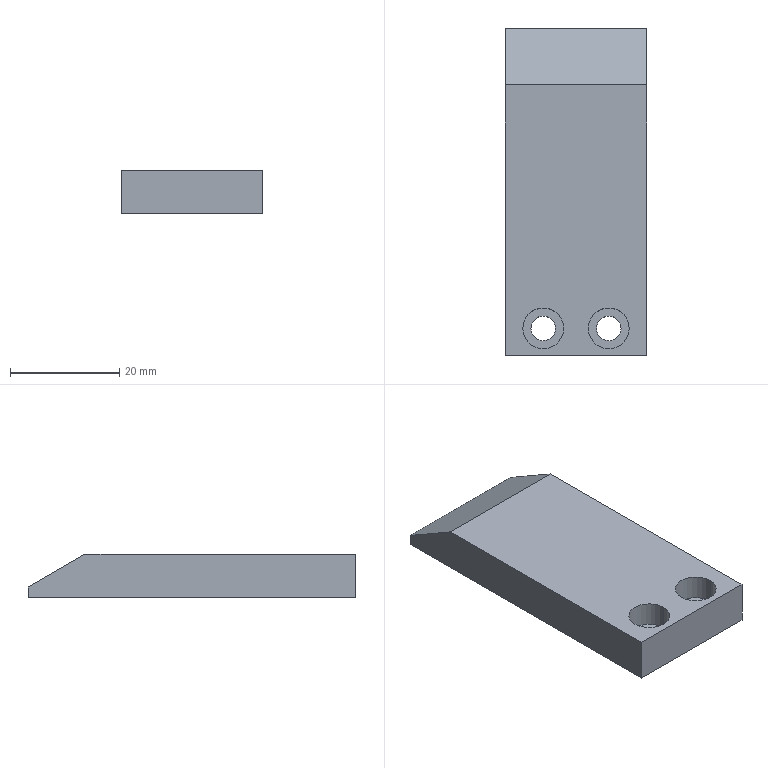Part | STEP file | CA-10-013Pusher Plate | 1 solid | 17 faces | box 26 x 60 x 8 mm | volume 11155 mm3 | plane 9 | cylinder 8 | commonest cylinder face diameters 4.5 x4 7.5 x4
STEP:
#1=CARTESIAN_POINT('',(0.,0.,0.));
#2=DIRECTION('',(0.,0.,1.));
#3=DIRECTION('',(1.,0.,0.));
#4=AXIS2_PLACEMENT_3D('',#1,#2,#3);
#5=CARTESIAN_POINT('',(9.75,-1.,-0.6));
#6=VERTEX_POINT('',#5);
#7=CARTESIAN_POINT('',(9.75,-1.,4.));
#8=VERTEX_POINT('',#7);
#9=CARTESIAN_POINT('',(9.75,-1.,4.));
#10=DIRECTION('',(0.,0.,1.));
#11=VECTOR('',#10,1.);
#12=LINE('',#9,#11);
#13=CARTESIAN_POINT('',(6.,-1.,4.));
#14=DIRECTION('',(0.,0.,1.));
#15=DIRECTION('',(1.,0.,0.));
#16=AXIS2_PLACEMENT_3D('',#13,#14,#15);
#17=CYLINDRICAL_SURFACE('',#16,3.75);
#18=CARTESIAN_POINT('',(6.283,0.));
#19=DIRECTION('',(0.,1.));
#20=VECTOR('',#19,1.);
#21=LINE('',#18,#20);
#22=(GEOMETRIC_REPRESENTATION_CONTEXT(2)PARAMETRIC_REPRESENTATION_CONTEXT()REPRESENTATION_CONTEXT('',''));
#23=DEFINITIONAL_REPRESENTATION('',(#21),#22);
#24=PCURVE('',#17,#23);
#25=CARTESIAN_POINT('',(6.,-1.,4.));
#26=DIRECTION('',(0.,0.,1.));
#27=DIRECTION('',(1.,0.,0.));
#28=AXIS2_PLACEMENT_3D('',#25,#26,#27);
#29=CYLINDRICAL_SURFACE('',#28,3.75);
#30=CARTESIAN_POINT('',(0.,0.));
#31=DIRECTION('',(0.,1.));
#32=VECTOR('',#31,1.);
#33=LINE('',#30,#32);
#34=(GEOMETRIC_REPRESENTATION_CONTEXT(2)PARAMETRIC_REPRESENTATION_CONTEXT()REPRESENTATION_CONTEXT('',''));
#35=DEFINITIONAL_REPRESENTATION('',(#33),#34);
#36=PCURVE('',#29,#35);
#37=SURFACE_CURVE('',#12,(#24,#36),.PCURVE_S1.);
#38=EDGE_CURVE('',#6,#8,#37,.T.);
#39=ORIENTED_EDGE('',*,*,#38,.T.);
#40=CARTESIAN_POINT('',(2.25,-1.,4.));
#41=VERTEX_POINT('',#40);
#42=CARTESIAN_POINT('',(6.,-1.,4.));
#43=DIRECTION('',(0.,0.,1.));
#44=DIRECTION('',(1.,0.,0.));
#45=AXIS2_PLACEMENT_3D('',#42,#43,#44);
#46=CIRCLE('',#45,3.75);
#47=CARTESIAN_POINT('',(0.,0.));
#48=DIRECTION('',(1.,0.));
#49=VECTOR('',#48,1.);
#50=LINE('',#47,#49);
#51=(GEOMETRIC_REPRESENTATION_CONTEXT(2)PARAMETRIC_REPRESENTATION_CONTEXT()REPRESENTATION_CONTEXT('',''));
#52=DEFINITIONAL_REPRESENTATION('',(#50),#51);
#53=PCURVE('',#17,#52);
#54=CARTESIAN_POINT('',(0.,0.,4.));
#55=DIRECTION('',(0.,0.,1.));
#56=DIRECTION('',(1.,0.,0.));
#57=AXIS2_PLACEMENT_3D('',#54,#55,#56);
#58=PLANE('',#57);
#59=CARTESIAN_POINT('',(6.,-1.));
#60=DIRECTION('',(1.,0.));
#61=AXIS2_PLACEMENT_2D('',#59,#60);
#62=CIRCLE('',#61,3.75);
#63=(GEOMETRIC_REPRESENTATION_CONTEXT(2)PARAMETRIC_REPRESENTATION_CONTEXT()REPRESENTATION_CONTEXT('',''));
#64=DEFINITIONAL_REPRESENTATION('',(#62),#63);
#65=PCURVE('',#58,#64);
#66=SURFACE_CURVE('',#46,(#53,#65),.PCURVE_S1.);
#67=EDGE_CURVE('',#41,#8,#66,.T.);
#68=ORIENTED_EDGE('',*,*,#67,.F.);
#69=CARTESIAN_POINT('',(2.25,-1.,-0.6));
#70=VERTEX_POINT('',#69);
#71=CARTESIAN_POINT('',(2.25,-1.,4.));
#72=DIRECTION('',(0.,0.,1.));
#73=VECTOR('',#72,1.);
#74=LINE('',#71,#73);
#75=CARTESIAN_POINT('',(3.142,0.));
#76=DIRECTION('',(0.,1.));
#77=VECTOR('',#76,1.);
#78=LINE('',#75,#77);
#79=(GEOMETRIC_REPRESENTATION_CONTEXT(2)PARAMETRIC_REPRESENTATION_CONTEXT()REPRESENTATION_CONTEXT('',''));
#80=DEFINITIONAL_REPRESENTATION('',(#78),#79);
#81=PCURVE('',#17,#80);
#82=CARTESIAN_POINT('',(3.142,0.));
#83=DIRECTION('',(0.,1.));
#84=VECTOR('',#83,1.);
#85=LINE('',#82,#84);
#86=(GEOMETRIC_REPRESENTATION_CONTEXT(2)PARAMETRIC_REPRESENTATION_CONTEXT()REPRESENTATION_CONTEXT('',''));
#87=DEFINITIONAL_REPRESENTATION('',(#85),#86);
#88=PCURVE('',#29,#87);
#89=SURFACE_CURVE('',#74,(#81,#88),.PCURVE_S1.);
#90=EDGE_CURVE('',#70,#41,#89,.T.);
#91=ORIENTED_EDGE('',*,*,#90,.F.);
#92=CARTESIAN_POINT('',(6.,-1.,-0.6));
#93=DIRECTION('',(0.,0.,1.));
#94=DIRECTION('',(1.,0.,0.));
#95=AXIS2_PLACEMENT_3D('',#92,#93,#94);
#96=CIRCLE('',#95,3.75);
#97=CARTESIAN_POINT('',(0.,-4.6));
#98=DIRECTION('',(1.,0.));
#99=VECTOR('',#98,1.);
#100=LINE('',#97,#99);
#101=(GEOMETRIC_REPRESENTATION_CONTEXT(2)PARAMETRIC_REPRESENTATION_CONTEXT()REPRESENTATION_CONTEXT('',''));
#102=DEFINITIONAL_REPRESENTATION('',(#100),#101);
#103=PCURVE('',#17,#102);
#104=CARTESIAN_POINT('',(8.25,-1.,-0.6));
#105=DIRECTION('',(0.,0.,-1.));
#106=DIRECTION('',(-1.,0.,0.));
#107=AXIS2_PLACEMENT_3D('',#104,#105,#106);
#108=PLANE('',#107);
#109=CARTESIAN_POINT('',(-1.5,0.));
#110=CARTESIAN_POINT('',(-1.5,6.495));
#111=CARTESIAN_POINT('',(4.125,3.248));
#112=CARTESIAN_POINT('',(9.75,0.));
#113=CARTESIAN_POINT('',(4.125,-3.248));
#114=CARTESIAN_POINT('',(-1.5,-6.495));
#115=CARTESIAN_POINT('',(-1.5,0.));
#116=(BOUNDED_CURVE()B_SPLINE_CURVE(2,(#109,#110,#111,#112,#113,#114,#115),.UNSPECIFIED.,.T.,.F.)B_SPLINE_CURVE_WITH_KNOTS((1,2,2,2,2,1),(-2.094,0.,2.094,4.189,6.283,8.378),.UNSPECIFIED.)CURVE()GEOMETRIC_REPRESENTATION_ITEM()RATIONAL_B_SPLINE_CURVE((1.,0.5,1.,0.5,1.,0.5,1.))REPRESENTATION_ITEM(''));
#117=(GEOMETRIC_REPRESENTATION_CONTEXT(2)PARAMETRIC_REPRESENTATION_CONTEXT()REPRESENTATION_CONTEXT('',''));
#118=DEFINITIONAL_REPRESENTATION('',(#116),#117);
#119=PCURVE('',#108,#118);
#120=SURFACE_CURVE('',#96,(#103,#119),.PCURVE_S1.);
#121=EDGE_CURVE('',#70,#6,#120,.T.);
#122=ORIENTED_EDGE('',*,*,#121,.T.);
#123=EDGE_LOOP('',(#39,#68,#91,#122));
#124=FACE_BOUND('',#123,.F.);
#125=ADVANCED_FACE('',(#124),#17,.F.);
#126=CARTESIAN_POINT('',(8.25,-1.,-4.));
#127=VERTEX_POINT('',#126);
#128=CARTESIAN_POINT('',(8.25,-1.,-0.6));
#129=VERTEX_POINT('',#128);
#130=CARTESIAN_POINT('',(8.25,-1.,4.));
#131=DIRECTION('',(0.,0.,1.));
#132=VECTOR('',#131,1.);
#133=LINE('',#130,#132);
#134=CARTESIAN_POINT('',(6.,-1.,4.));
#135=DIRECTION('',(0.,0.,1.));
#136=DIRECTION('',(1.,0.,0.));
#137=AXIS2_PLACEMENT_3D('',#134,#135,#136);
#138=CYLINDRICAL_SURFACE('',#137,2.25);
#139=CARTESIAN_POINT('',(6.283,0.));
#140=DIRECTION('',(0.,1.));
#141=VECTOR('',#140,1.);
#142=LINE('',#139,#141);
#143=(GEOMETRIC_REPRESENTATION_CONTEXT(2)PARAMETRIC_REPRESENTATION_CONTEXT()REPRESENTATION_CONTEXT('',''));
#144=DEFINITIONAL_REPRESENTATION('',(#142),#143);
#145=PCURVE('',#138,#144);
#146=CARTESIAN_POINT('',(6.,-1.,4.));
#147=DIRECTION('',(0.,0.,1.));
#148=DIRECTION('',(1.,0.,0.));
#149=AXIS2_PLACEMENT_3D('',#146,#147,#148);
#150=CYLINDRICAL_SURFACE('',#149,2.25);
#151=CARTESIAN_POINT('',(0.,0.));
#152=DIRECTION('',(0.,1.));
#153=VECTOR('',#152,1.);
#154=LINE('',#151,#153);
#155=(GEOMETRIC_REPRESENTATION_CONTEXT(2)PARAMETRIC_REPRESENTATION_CONTEXT()REPRESENTATION_CONTEXT('',''));
#156=DEFINITIONAL_REPRESENTATION('',(#154),#155);
#157=PCURVE('',#150,#156);
#158=SURFACE_CURVE('',#133,(#145,#157),.PCURVE_S1.);
#159=EDGE_CURVE('',#127,#129,#158,.T.);
#160=ORIENTED_EDGE('',*,*,#159,.T.);
#161=CARTESIAN_POINT('',(3.75,-1.,-0.6));
#162=VERTEX_POINT('',#161);
#163=CARTESIAN_POINT('',(6.,-1.,-0.6));
#164=DIRECTION('',(0.,0.,1.));
#165=DIRECTION('',(1.,0.,0.));
#166=AXIS2_PLACEMENT_3D('',#163,#164,#165);
#167=CIRCLE('',#166,2.25);
#168=CARTESIAN_POINT('',(0.,-4.6));
#169=DIRECTION('',(1.,0.));
#170=VECTOR('',#169,1.);
#171=LINE('',#168,#170);
#172=(GEOMETRIC_REPRESENTATION_CONTEXT(2)PARAMETRIC_REPRESENTATION_CONTEXT()REPRESENTATION_CONTEXT('',''));
#173=DEFINITIONAL_REPRESENTATION('',(#171),#172);
#174=PCURVE('',#138,#173);
#175=CARTESIAN_POINT('',(0.,0.));
#176=CARTESIAN_POINT('',(0.,3.897));
#177=CARTESIAN_POINT('',(3.375,1.949));
#178=CARTESIAN_POINT('',(6.75,0.));
#179=CARTESIAN_POINT('',(3.375,-1.949));
#180=CARTESIAN_POINT('',(0.,-3.897));
#181=CARTESIAN_POINT('',(0.,0.));
#182=(BOUNDED_CURVE()B_SPLINE_CURVE(2,(#175,#176,#177,#178,#179,#180,#181),.UNSPECIFIED.,.T.,.F.)B_SPLINE_CURVE_WITH_KNOTS((1,2,2,2,2,1),(-2.094,0.,2.094,4.189,6.283,8.378),.UNSPECIFIED.)CURVE()GEOMETRIC_REPRESENTATION_ITEM()RATIONAL_B_SPLINE_CURVE((1.,0.5,1.,0.5,1.,0.5,1.))REPRESENTATION_ITEM(''));
#183=(GEOMETRIC_REPRESENTATION_CONTEXT(2)PARAMETRIC_REPRESENTATION_CONTEXT()REPRESENTATION_CONTEXT('',''));
#184=DEFINITIONAL_REPRESENTATION('',(#182),#183);
#185=PCURVE('',#108,#184);
#186=SURFACE_CURVE('',#167,(#174,#185),.PCURVE_S1.);
#187=EDGE_CURVE('',#162,#129,#186,.T.);
#188=ORIENTED_EDGE('',*,*,#187,.F.);
#189=CARTESIAN_POINT('',(3.75,-1.,-4.));
#190=VERTEX_POINT('',#189);
#191=CARTESIAN_POINT('',(3.75,-1.,4.));
#192=DIRECTION('',(0.,0.,1.));
#193=VECTOR('',#192,1.);
#194=LINE('',#191,#193);
#195=CARTESIAN_POINT('',(3.142,0.));
#196=DIRECTION('',(0.,1.));
#197=VECTOR('',#196,1.);
#198=LINE('',#195,#197);
#199=(GEOMETRIC_REPRESENTATION_CONTEXT(2)PARAMETRIC_REPRESENTATION_CONTEXT()REPRESENTATION_CONTEXT('',''));
#200=DEFINITIONAL_REPRESENTATION('',(#198),#199);
#201=PCURVE('',#138,#200);
#202=CARTESIAN_POINT('',(3.142,0.));
#203=DIRECTION('',(0.,1.));
#204=VECTOR('',#203,1.);
#205=LINE('',#202,#204);
#206=(GEOMETRIC_REPRESENTATION_CONTEXT(2)PARAMETRIC_REPRESENTATION_CONTEXT()REPRESENTATION_CONTEXT('',''));
#207=DEFINITIONAL_REPRESENTATION('',(#205),#206);
#208=PCURVE('',#150,#207);
#209=SURFACE_CURVE('',#194,(#201,#208),.PCURVE_S1.);
#210=EDGE_CURVE('',#190,#162,#209,.T.);
#211=ORIENTED_EDGE('',*,*,#210,.F.);
#212=CARTESIAN_POINT('',(6.,-1.,-4.));
#213=DIRECTION('',(0.,0.,1.));
#214=DIRECTION('',(1.,0.,0.));
#215=AXIS2_PLACEMENT_3D('',#212,#213,#214);
#216=CIRCLE('',#215,2.25);
#217=CARTESIAN_POINT('',(0.,-8.));
#218=DIRECTION('',(1.,0.));
#219=VECTOR('',#218,1.);
#220=LINE('',#217,#219);
#221=(GEOMETRIC_REPRESENTATION_CONTEXT(2)PARAMETRIC_REPRESENTATION_CONTEXT()REPRESENTATION_CONTEXT('',''));
#222=DEFINITIONAL_REPRESENTATION('',(#220),#221);
#223=PCURVE('',#138,#222);
#224=CARTESIAN_POINT('',(0.,0.,-4.));
#225=DIRECTION('',(0.,0.,1.));
#226=DIRECTION('',(1.,0.,0.));
#227=AXIS2_PLACEMENT_3D('',#224,#225,#226);
#228=PLANE('',#227);
#229=CARTESIAN_POINT('',(6.,-1.));
#230=DIRECTION('',(1.,0.));
#231=AXIS2_PLACEMENT_2D('',#229,#230);
#232=CIRCLE('',#231,2.25);
#233=(GEOMETRIC_REPRESENTATION_CONTEXT(2)PARAMETRIC_REPRESENTATION_CONTEXT()REPRESENTATION_CONTEXT('',''));
#234=DEFINITIONAL_REPRESENTATION('',(#232),#233);
#235=PCURVE('',#228,#234);
#236=SURFACE_CURVE('',#216,(#223,#235),.PCURVE_S1.);
#237=EDGE_CURVE('',#190,#127,#236,.T.);
#238=ORIENTED_EDGE('',*,*,#237,.T.);
#239=EDGE_LOOP('',(#160,#188,#211,#238));
#240=FACE_BOUND('',#239,.F.);
#241=ADVANCED_FACE('',(#240),#138,.F.);
#242=CARTESIAN_POINT('',(-2.25,-1.,-0.6));
#243=VERTEX_POINT('',#242);
#244=CARTESIAN_POINT('',(-2.25,-1.,4.));
#245=VERTEX_POINT('',#244);
#246=CARTESIAN_POINT('',(-2.25,-1.,4.));
#247=DIRECTION('',(0.,0.,1.));
#248=VECTOR('',#247,1.);
#249=LINE('',#246,#248);
#250=CARTESIAN_POINT('',(-6.,-1.,4.));
#251=DIRECTION('',(0.,0.,1.));
#252=DIRECTION('',(1.,0.,0.));
#253=AXIS2_PLACEMENT_3D('',#250,#251,#252);
#254=CYLINDRICAL_SURFACE('',#253,3.75);
#255=CARTESIAN_POINT('',(6.283,0.));
#256=DIRECTION('',(0.,1.));
#257=VECTOR('',#256,1.);
#258=LINE('',#255,#257);
#259=(GEOMETRIC_REPRESENTATION_CONTEXT(2)PARAMETRIC_REPRESENTATION_CONTEXT()REPRESENTATION_CONTEXT('',''));
#260=DEFINITIONAL_REPRESENTATION('',(#258),#259);
#261=PCURVE('',#254,#260);
#262=CARTESIAN_POINT('',(-6.,-1.,4.));
#263=DIRECTION('',(0.,0.,1.));
#264=DIRECTION('',(1.,0.,0.));
#265=AXIS2_PLACEMENT_3D('',#262,#263,#264);
#266=CYLINDRICAL_SURFACE('',#265,3.75);
#267=CARTESIAN_POINT('',(0.,0.));
#268=DIRECTION('',(0.,1.));
#269=VECTOR('',#268,1.);
#270=LINE('',#267,#269);
#271=(GEOMETRIC_REPRESENTATION_CONTEXT(2)PARAMETRIC_REPRESENTATION_CONTEXT()REPRESENTATION_CONTEXT('',''));
#272=DEFINITIONAL_REPRESENTATION('',(#270),#271);
#273=PCURVE('',#266,#272);
#274=SURFACE_CURVE('',#249,(#261,#273),.PCURVE_S1.);
#275=EDGE_CURVE('',#243,#245,#274,.T.);
#276=ORIENTED_EDGE('',*,*,#275,.T.);
#277=CARTESIAN_POINT('',(-9.75,-1.,4.));
#278=VERTEX_POINT('',#277);
#279=CARTESIAN_POINT('',(-6.,-1.,4.));
#280=DIRECTION('',(0.,0.,1.));
#281=DIRECTION('',(1.,0.,0.));
#282=AXIS2_PLACEMENT_3D('',#279,#280,#281);
#283=CIRCLE('',#282,3.75);
#284=CARTESIAN_POINT('',(0.,0.));
#285=DIRECTION('',(1.,0.));
#286=VECTOR('',#285,1.);
#287=LINE('',#284,#286);
#288=(GEOMETRIC_REPRESENTATION_CONTEXT(2)PARAMETRIC_REPRESENTATION_CONTEXT()REPRESENTATION_CONTEXT('',''));
#289=DEFINITIONAL_REPRESENTATION('',(#287),#288);
#290=PCURVE('',#254,#289);
#291=CARTESIAN_POINT('',(-6.,-1.));
#292=DIRECTION('',(1.,0.));
#293=AXIS2_PLACEMENT_2D('',#291,#292);
#294=CIRCLE('',#293,3.75);
#295=(GEOMETRIC_REPRESENTATION_CONTEXT(2)PARAMETRIC_REPRESENTATION_CONTEXT()REPRESENTATION_CONTEXT('',''));
#296=DEFINITIONAL_REPRESENTATION('',(#294),#295);
#297=PCURVE('',#58,#296);
#298=SURFACE_CURVE('',#283,(#290,#297),.PCURVE_S1.);
#299=EDGE_CURVE('',#278,#245,#298,.T.);
#300=ORIENTED_EDGE('',*,*,#299,.F.);
#301=CARTESIAN_POINT('',(-9.75,-1.,-0.6));
#302=VERTEX_POINT('',#301);
#303=CARTESIAN_POINT('',(-9.75,-1.,4.));
#304=DIRECTION('',(0.,0.,1.));
#305=VECTOR('',#304,1.);
#306=LINE('',#303,#305);
#307=CARTESIAN_POINT('',(3.142,0.));
#308=DIRECTION('',(0.,1.));
#309=VECTOR('',#308,1.);
#310=LINE('',#307,#309);
#311=(GEOMETRIC_REPRESENTATION_CONTEXT(2)PARAMETRIC_REPRESENTATION_CONTEXT()REPRESENTATION_CONTEXT('',''));
#312=DEFINITIONAL_REPRESENTATION('',(#310),#311);
#313=PCURVE('',#254,#312);
#314=CARTESIAN_POINT('',(3.142,0.));
#315=DIRECTION('',(0.,1.));
#316=VECTOR('',#315,1.);
#317=LINE('',#314,#316);
#318=(GEOMETRIC_REPRESENTATION_CONTEXT(2)PARAMETRIC_REPRESENTATION_CONTEXT()REPRESENTATION_CONTEXT('',''));
#319=DEFINITIONAL_REPRESENTATION('',(#317),#318);
#320=PCURVE('',#266,#319);
#321=SURFACE_CURVE('',#306,(#313,#320),.PCURVE_S1.);
#322=EDGE_CURVE('',#302,#278,#321,.T.);
#323=ORIENTED_EDGE('',*,*,#322,.F.);
#324=CARTESIAN_POINT('',(-6.,-1.,-0.6));
#325=DIRECTION('',(0.,0.,1.));
#326=DIRECTION('',(1.,0.,0.));
#327=AXIS2_PLACEMENT_3D('',#324,#325,#326);
#328=CIRCLE('',#327,3.75);
#329=CARTESIAN_POINT('',(0.,-4.6));
#330=DIRECTION('',(1.,0.));
#331=VECTOR('',#330,1.);
#332=LINE('',#329,#331);
#333=(GEOMETRIC_REPRESENTATION_CONTEXT(2)PARAMETRIC_REPRESENTATION_CONTEXT()REPRESENTATION_CONTEXT('',''));
#334=DEFINITIONAL_REPRESENTATION('',(#332),#333);
#335=PCURVE('',#254,#334);
#336=CARTESIAN_POINT('',(-3.75,-1.,-0.6));
#337=DIRECTION('',(0.,0.,-1.));
#338=DIRECTION('',(-1.,0.,0.));
#339=AXIS2_PLACEMENT_3D('',#336,#337,#338);
#340=PLANE('',#339);
#341=CARTESIAN_POINT('',(-1.5,0.));
#342=CARTESIAN_POINT('',(-1.5,6.495));
#343=CARTESIAN_POINT('',(4.125,3.248));
#344=CARTESIAN_POINT('',(9.75,0.));
#345=CARTESIAN_POINT('',(4.125,-3.248));
#346=CARTESIAN_POINT('',(-1.5,-6.495));
#347=CARTESIAN_POINT('',(-1.5,0.));
#348=(BOUNDED_CURVE()B_SPLINE_CURVE(2,(#341,#342,#343,#344,#345,#346,#347),.UNSPECIFIED.,.T.,.F.)B_SPLINE_CURVE_WITH_KNOTS((1,2,2,2,2,1),(-2.094,0.,2.094,4.189,6.283,8.378),.UNSPECIFIED.)CURVE()GEOMETRIC_REPRESENTATION_ITEM()RATIONAL_B_SPLINE_CURVE((1.,0.5,1.,0.5,1.,0.5,1.))REPRESENTATION_ITEM(''));
#349=(GEOMETRIC_REPRESENTATION_CONTEXT(2)PARAMETRIC_REPRESENTATION_CONTEXT()REPRESENTATION_CONTEXT('',''));
#350=DEFINITIONAL_REPRESENTATION('',(#348),#349);
#351=PCURVE('',#340,#350);
#352=SURFACE_CURVE('',#328,(#335,#351),.PCURVE_S1.);
#353=EDGE_CURVE('',#302,#243,#352,.T.);
#354=ORIENTED_EDGE('',*,*,#353,.T.);
#355=EDGE_LOOP('',(#276,#300,#323,#354));
#356=FACE_BOUND('',#355,.F.);
#357=ADVANCED_FACE('',(#356),#254,.F.);
#358=CARTESIAN_POINT('',(-3.75,-1.,-4.));
#359=VERTEX_POINT('',#358);
#360=CARTESIAN_POINT('',(-3.75,-1.,-0.6));
#361=VERTEX_POINT('',#360);
#362=CARTESIAN_POINT('',(-3.75,-1.,4.));
#363=DIRECTION('',(0.,0.,1.));
#364=VECTOR('',#363,1.);
#365=LINE('',#362,#364);
#366=CARTESIAN_POINT('',(-6.,-1.,4.));
#367=DIRECTION('',(0.,0.,1.));
#368=DIRECTION('',(1.,0.,0.));
#369=AXIS2_PLACEMENT_3D('',#366,#367,#368);
#370=CYLINDRICAL_SURFACE('',#369,2.25);
#371=CARTESIAN_POINT('',(6.283,0.));
#372=DIRECTION('',(0.,1.));
#373=VECTOR('',#372,1.);
#374=LINE('',#371,#373);
#375=(GEOMETRIC_REPRESENTATION_CONTEXT(2)PARAMETRIC_REPRESENTATION_CONTEXT()REPRESENTATION_CONTEXT('',''));
#376=DEFINITIONAL_REPRESENTATION('',(#374),#375);
#377=PCURVE('',#370,#376);
#378=CARTESIAN_POINT('',(-6.,-1.,4.));
#379=DIRECTION('',(0.,0.,1.));
#380=DIRECTION('',(1.,0.,0.));
#381=AXIS2_PLACEMENT_3D('',#378,#379,#380);
#382=CYLINDRICAL_SURFACE('',#381,2.25);
#383=CARTESIAN_POINT('',(0.,0.));
#384=DIRECTION('',(0.,1.));
#385=VECTOR('',#384,1.);
#386=LINE('',#383,#385);
#387=(GEOMETRIC_REPRESENTATION_CONTEXT(2)PARAMETRIC_REPRESENTATION_CONTEXT()REPRESENTATION_CONTEXT('',''));
#388=DEFINITIONAL_REPRESENTATION('',(#386),#387);
#389=PCURVE('',#382,#388);
#390=SURFACE_CURVE('',#365,(#377,#389),.PCURVE_S1.);
#391=EDGE_CURVE('',#359,#361,#390,.T.);
#392=ORIENTED_EDGE('',*,*,#391,.T.);
#393=CARTESIAN_POINT('',(-8.25,-1.,-0.6));
#394=VERTEX_POINT('',#393);
#395=CARTESIAN_POINT('',(-6.,-1.,-0.6));
#396=DIRECTION('',(0.,0.,1.));
#397=DIRECTION('',(1.,0.,0.));
#398=AXIS2_PLACEMENT_3D('',#395,#396,#397);
#399=CIRCLE('',#398,2.25);
#400=CARTESIAN_POINT('',(0.,-4.6));
#401=DIRECTION('',(1.,0.));
#402=VECTOR('',#401,1.);
#403=LINE('',#400,#402);
#404=(GEOMETRIC_REPRESENTATION_CONTEXT(2)PARAMETRIC_REPRESENTATION_CONTEXT()REPRESENTATION_CONTEXT('',''));
#405=DEFINITIONAL_REPRESENTATION('',(#403),#404);
#406=PCURVE('',#370,#405);
#407=CARTESIAN_POINT('',(0.,0.));
#408=CARTESIAN_POINT('',(0.,3.897));
#409=CARTESIAN_POINT('',(3.375,1.949));
#410=CARTESIAN_POINT('',(6.75,0.));
#411=CARTESIAN_POINT('',(3.375,-1.949));
#412=CARTESIAN_POINT('',(0.,-3.897));
#413=CARTESIAN_POINT('',(0.,0.));
#414=(BOUNDED_CURVE()B_SPLINE_CURVE(2,(#407,#408,#409,#410,#411,#412,#413),.UNSPECIFIED.,.T.,.F.)B_SPLINE_CURVE_WITH_KNOTS((1,2,2,2,2,1),(-2.094,0.,2.094,4.189,6.283,8.378),.UNSPECIFIED.)CURVE()GEOMETRIC_REPRESENTATION_ITEM()RATIONAL_B_SPLINE_CURVE((1.,0.5,1.,0.5,1.,0.5,1.))REPRESENTATION_ITEM(''));
#415=(GEOMETRIC_REPRESENTATION_CONTEXT(2)PARAMETRIC_REPRESENTATION_CONTEXT()REPRESENTATION_CONTEXT('',''));
#416=DEFINITIONAL_REPRESENTATION('',(#414),#415);
#417=PCURVE('',#340,#416);
#418=SURFACE_CURVE('',#399,(#406,#417),.PCURVE_S1.);
#419=EDGE_CURVE('',#394,#361,#418,.T.);
#420=ORIENTED_EDGE('',*,*,#419,.F.);
#421=CARTESIAN_POINT('',(-8.25,-1.,-4.));
#422=VERTEX_POINT('',#421);
#423=CARTESIAN_POINT('',(-8.25,-1.,4.));
#424=DIRECTION('',(0.,0.,1.));
#425=VECTOR('',#424,1.);
#426=LINE('',#423,#425);
#427=CARTESIAN_POINT('',(3.142,0.));
#428=DIRECTION('',(0.,1.));
#429=VECTOR('',#428,1.);
#430=LINE('',#427,#429);
#431=(GEOMETRIC_REPRESENTATION_CONTEXT(2)PARAMETRIC_REPRESENTATION_CONTEXT()REPRESENTATION_CONTEXT('',''));
#432=DEFINITIONAL_REPRESENTATION('',(#430),#431);
#433=PCURVE('',#370,#432);
#434=CARTESIAN_POINT('',(3.142,0.));
#435=DIRECTION('',(0.,1.));
#436=VECTOR('',#435,1.);
#437=LINE('',#434,#436);
#438=(GEOMETRIC_REPRESENTATION_CONTEXT(2)PARAMETRIC_REPRESENTATION_CONTEXT()REPRESENTATION_CONTEXT('',''));
#439=DEFINITIONAL_REPRESENTATION('',(#437),#438);
#440=PCURVE('',#382,#439);
#441=SURFACE_CURVE('',#426,(#433,#440),.PCURVE_S1.);
#442=EDGE_CURVE('',#422,#394,#441,.T.);
#443=ORIENTED_EDGE('',*,*,#442,.F.);
#444=CARTESIAN_POINT('',(-6.,-1.,-4.));
#445=DIRECTION('',(0.,0.,1.));
#446=DIRECTION('',(1.,0.,0.));
#447=AXIS2_PLACEMENT_3D('',#444,#445,#446);
#448=CIRCLE('',#447,2.25);
#449=CARTESIAN_POINT('',(0.,-8.));
#450=DIRECTION('',(1.,0.));
#451=VECTOR('',#450,1.);
#452=LINE('',#449,#451);
#453=(GEOMETRIC_REPRESENTATION_CONTEXT(2)PARAMETRIC_REPRESENTATION_CONTEXT()REPRESENTATION_CONTEXT('',''));
#454=DEFINITIONAL_REPRESENTATION('',(#452),#453);
#455=PCURVE('',#370,#454);
#456=CARTESIAN_POINT('',(-6.,-1.));
#457=DIRECTION('',(1.,0.));
#458=AXIS2_PLACEMENT_2D('',#456,#457);
#459=CIRCLE('',#458,2.25);
#460=(GEOMETRIC_REPRESENTATION_CONTEXT(2)PARAMETRIC_REPRESENTATION_CONTEXT()REPRESENTATION_CONTEXT('',''));
#461=DEFINITIONAL_REPRESENTATION('',(#459),#460);
#462=PCURVE('',#228,#461);
#463=SURFACE_CURVE('',#448,(#455,#462),.PCURVE_S1.);
#464=EDGE_CURVE('',#422,#359,#463,.T.);
#465=ORIENTED_EDGE('',*,*,#464,.T.);
#466=EDGE_LOOP('',(#392,#420,#443,#465));
#467=FACE_BOUND('',#466,.F.);
#468=ADVANCED_FACE('',(#467),#370,.F.);
#469=CARTESIAN_POINT('',(-13.,43.608,4.));
#470=VERTEX_POINT('',#469);
#471=CARTESIAN_POINT('',(-13.,-6.,4.));
#472=VERTEX_POINT('',#471);
#473=CARTESIAN_POINT('',(-13.,54.,4.));
#474=DIRECTION('',(0.,-1.,0.));
#475=VECTOR('',#474,1.);
#476=LINE('',#473,#475);
#477=CARTESIAN_POINT('',(-13.,54.,4.));
#478=DIRECTION('',(1.,0.,0.));
#479=DIRECTION('',(0.,1.,0.));
#480=AXIS2_PLACEMENT_3D('',#477,#478,#479);
#481=PLANE('',#480);
#482=CARTESIAN_POINT('',(0.,0.));
#483=DIRECTION('',(-1.,0.));
#484=VECTOR('',#483,1.);
#485=LINE('',#482,#484);
#486=(GEOMETRIC_REPRESENTATION_CONTEXT(2)PARAMETRIC_REPRESENTATION_CONTEXT()REPRESENTATION_CONTEXT('',''));
#487=DEFINITIONAL_REPRESENTATION('',(#485),#486);
#488=PCURVE('',#481,#487);
#489=CARTESIAN_POINT('',(-13.,54.));
#490=DIRECTION('',(0.,-1.));
#491=VECTOR('',#490,1.);
#492=LINE('',#489,#491);
#493=(GEOMETRIC_REPRESENTATION_CONTEXT(2)PARAMETRIC_REPRESENTATION_CONTEXT()REPRESENTATION_CONTEXT('',''));
#494=DEFINITIONAL_REPRESENTATION('',(#492),#493);
#495=PCURVE('',#58,#494);
#496=SURFACE_CURVE('',#476,(#488,#495),.PCURVE_S1.);
#497=EDGE_CURVE('',#470,#472,#496,.T.);
#498=ORIENTED_EDGE('',*,*,#497,.F.);
#499=CARTESIAN_POINT('',(-13.,54.,-2.));
#500=VERTEX_POINT('',#499);
#501=CARTESIAN_POINT('',(-13.,43.608,4.));
#502=DIRECTION('',(0.,0.866,-0.5));
#503=VECTOR('',#502,1.);
#504=LINE('',#501,#503);
#505=CARTESIAN_POINT('',(-10.392,0.));
#506=DIRECTION('',(0.866,-0.5));
#507=VECTOR('',#506,1.);
#508=LINE('',#505,#507);
#509=(GEOMETRIC_REPRESENTATION_CONTEXT(2)PARAMETRIC_REPRESENTATION_CONTEXT()REPRESENTATION_CONTEXT('',''));
#510=DEFINITIONAL_REPRESENTATION('',(#508),#509);
#511=PCURVE('',#481,#510);
#512=CARTESIAN_POINT('',(0.,43.608,4.));
#513=DIRECTION('',(0.,0.5,0.866));
#514=DIRECTION('',(1.,0.,0.));
#515=AXIS2_PLACEMENT_3D('',#512,#513,#514);
#516=PLANE('',#515);
#517=CARTESIAN_POINT('',(-13.,0.));
#518=DIRECTION('',(0.,1.));
#519=VECTOR('',#518,1.);
#520=LINE('',#517,#519);
#521=(GEOMETRIC_REPRESENTATION_CONTEXT(2)PARAMETRIC_REPRESENTATION_CONTEXT()REPRESENTATION_CONTEXT('',''));
#522=DEFINITIONAL_REPRESENTATION('',(#520),#521);
#523=PCURVE('',#516,#522);
#524=SURFACE_CURVE('',#504,(#511,#523),.PCURVE_S1.);
#525=EDGE_CURVE('',#470,#500,#524,.T.);
#526=ORIENTED_EDGE('',*,*,#525,.T.);
#527=CARTESIAN_POINT('',(-13.,54.,-4.));
#528=VERTEX_POINT('',#527);
#529=CARTESIAN_POINT('',(-13.,54.,4.));
#530=DIRECTION('',(0.,0.,-1.));
#531=VECTOR('',#530,1.);
#532=LINE('',#529,#531);
#533=CARTESIAN_POINT('',(0.,0.));
#534=DIRECTION('',(0.,-1.));
#535=VECTOR('',#534,1.);
#536=LINE('',#533,#535);
#537=(GEOMETRIC_REPRESENTATION_CONTEXT(2)PARAMETRIC_REPRESENTATION_CONTEXT()REPRESENTATION_CONTEXT('',''));
#538=DEFINITIONAL_REPRESENTATION('',(#536),#537);
#539=PCURVE('',#481,#538);
#540=CARTESIAN_POINT('',(-13.,54.,4.));
#541=DIRECTION('',(0.,-1.,0.));
#542=DIRECTION('',(0.,0.,-1.));
#543=AXIS2_PLACEMENT_3D('',#540,#541,#542);
#544=PLANE('',#543);
#545=CARTESIAN_POINT('',(0.,0.));
#546=DIRECTION('',(1.,0.));
#547=VECTOR('',#546,1.);
#548=LINE('',#545,#547);
#549=(GEOMETRIC_REPRESENTATION_CONTEXT(2)PARAMETRIC_REPRESENTATION_CONTEXT()REPRESENTATION_CONTEXT('',''));
#550=DEFINITIONAL_REPRESENTATION('',(#548),#549);
#551=PCURVE('',#544,#550);
#552=SURFACE_CURVE('',#532,(#539,#551),.PCURVE_S1.);
#553=EDGE_CURVE('',#500,#528,#552,.T.);
#554=ORIENTED_EDGE('',*,*,#553,.T.);
#555=CARTESIAN_POINT('',(-13.,-6.,-4.));
#556=VERTEX_POINT('',#555);
#557=CARTESIAN_POINT('',(-13.,54.,-4.));
#558=DIRECTION('',(0.,-1.,0.));
#559=VECTOR('',#558,1.);
#560=LINE('',#557,#559);
#561=CARTESIAN_POINT('',(0.,-8.));
#562=DIRECTION('',(-1.,0.));
#563=VECTOR('',#562,1.);
#564=LINE('',#561,#563);
#565=(GEOMETRIC_REPRESENTATION_CONTEXT(2)PARAMETRIC_REPRESENTATION_CONTEXT()REPRESENTATION_CONTEXT('',''));
#566=DEFINITIONAL_REPRESENTATION('',(#564),#565);
#567=PCURVE('',#481,#566);
#568=CARTESIAN_POINT('',(-13.,54.));
#569=DIRECTION('',(0.,-1.));
#570=VECTOR('',#569,1.);
#571=LINE('',#568,#570);
#572=(GEOMETRIC_REPRESENTATION_CONTEXT(2)PARAMETRIC_REPRESENTATION_CONTEXT()REPRESENTATION_CONTEXT('',''));
#573=DEFINITIONAL_REPRESENTATION('',(#571),#572);
#574=PCURVE('',#228,#573);
#575=SURFACE_CURVE('',#560,(#567,#574),.PCURVE_S1.);
#576=EDGE_CURVE('',#528,#556,#575,.T.);
#577=ORIENTED_EDGE('',*,*,#576,.T.);
#578=CARTESIAN_POINT('',(-13.,-6.,4.));
#579=DIRECTION('',(0.,0.,-1.));
#580=VECTOR('',#579,1.);
#581=LINE('',#578,#580);
#582=CARTESIAN_POINT('',(-60.,0.));
#583=DIRECTION('',(0.,-1.));
#584=VECTOR('',#583,1.);
#585=LINE('',#582,#584);
#586=(GEOMETRIC_REPRESENTATION_CONTEXT(2)PARAMETRIC_REPRESENTATION_CONTEXT()REPRESENTATION_CONTEXT('',''));
#587=DEFINITIONAL_REPRESENTATION('',(#585),#586);
#588=PCURVE('',#481,#587);
#589=CARTESIAN_POINT('',(-13.,-6.,4.));
#590=DIRECTION('',(0.,1.,0.));
#591=DIRECTION('',(-1.,0.,0.));
#592=AXIS2_PLACEMENT_3D('',#589,#590,#591);
#593=PLANE('',#592);
#594=CARTESIAN_POINT('',(0.,0.));
#595=DIRECTION('',(0.,-1.));
#596=VECTOR('',#595,1.);
#597=LINE('',#594,#596);
#598=(GEOMETRIC_REPRESENTATION_CONTEXT(2)PARAMETRIC_REPRESENTATION_CONTEXT()REPRESENTATION_CONTEXT('',''));
#599=DEFINITIONAL_REPRESENTATION('',(#597),#598);
#600=PCURVE('',#593,#599);
#601=SURFACE_CURVE('',#581,(#588,#600),.PCURVE_S1.);
#602=EDGE_CURVE('',#472,#556,#601,.T.);
#603=ORIENTED_EDGE('',*,*,#602,.F.);
#604=EDGE_LOOP('',(#498,#526,#554,#577,#603));
#605=FACE_BOUND('',#604,.T.);
#606=ADVANCED_FACE('',(#605),#481,.F.);
#607=CARTESIAN_POINT('',(13.,-6.,-4.));
#608=VERTEX_POINT('',#607);
#609=CARTESIAN_POINT('',(-13.,-6.,-4.));
#610=DIRECTION('',(1.,0.,0.));
#611=VECTOR('',#610,1.);
#612=LINE('',#609,#611);
#613=CARTESIAN_POINT('',(0.,-8.));
#614=DIRECTION('',(-1.,0.));
#615=VECTOR('',#614,1.);
#616=LINE('',#613,#615);
#617=(GEOMETRIC_REPRESENTATION_CONTEXT(2)PARAMETRIC_REPRESENTATION_CONTEXT()REPRESENTATION_CONTEXT('',''));
#618=DEFINITIONAL_REPRESENTATION('',(#616),#617);
#619=PCURVE('',#593,#618);
#620=CARTESIAN_POINT('',(-13.,-6.));
#621=DIRECTION('',(1.,0.));
#622=VECTOR('',#621,1.);
#623=LINE('',#620,#622);
#624=(GEOMETRIC_REPRESENTATION_CONTEXT(2)PARAMETRIC_REPRESENTATION_CONTEXT()REPRESENTATION_CONTEXT('',''));
#625=DEFINITIONAL_REPRESENTATION('',(#623),#624);
#626=PCURVE('',#228,#625);
#627=SURFACE_CURVE('',#612,(#619,#626),.PCURVE_S1.);
#628=EDGE_CURVE('',#556,#608,#627,.T.);
#629=ORIENTED_EDGE('',*,*,#628,.T.);
#630=CARTESIAN_POINT('',(13.,-6.,4.));
#631=VERTEX_POINT('',#630);
#632=CARTESIAN_POINT('',(13.,-6.,4.));
#633=DIRECTION('',(0.,0.,-1.));
#634=VECTOR('',#633,1.);
#635=LINE('',#632,#634);
#636=CARTESIAN_POINT('',(-26.,0.));
#637=DIRECTION('',(0.,-1.));
#638=VECTOR('',#637,1.);
#639=LINE('',#636,#638);
#640=(GEOMETRIC_REPRESENTATION_CONTEXT(2)PARAMETRIC_REPRESENTATION_CONTEXT()REPRESENTATION_CONTEXT('',''));
#641=DEFINITIONAL_REPRESENTATION('',(#639),#640);
#642=PCURVE('',#593,#641);
#643=CARTESIAN_POINT('',(13.,54.,4.));
#644=DIRECTION('',(-1.,0.,0.));
#645=DIRECTION('',(0.,-1.,0.));
#646=AXIS2_PLACEMENT_3D('',#643,#644,#645);
#647=PLANE('',#646);
#648=CARTESIAN_POINT('',(60.,0.));
#649=DIRECTION('',(0.,-1.));
#650=VECTOR('',#649,1.);
#651=LINE('',#648,#650);
#652=(GEOMETRIC_REPRESENTATION_CONTEXT(2)PARAMETRIC_REPRESENTATION_CONTEXT()REPRESENTATION_CONTEXT('',''));
#653=DEFINITIONAL_REPRESENTATION('',(#651),#652);
#654=PCURVE('',#647,#653);
#655=SURFACE_CURVE('',#635,(#642,#654),.PCURVE_S1.);
#656=EDGE_CURVE('',#631,#608,#655,.T.);
#657=ORIENTED_EDGE('',*,*,#656,.F.);
#658=CARTESIAN_POINT('',(-13.,-6.,4.));
#659=DIRECTION('',(1.,0.,0.));
#660=VECTOR('',#659,1.);
#661=LINE('',#658,#660);
#662=CARTESIAN_POINT('',(0.,0.));
#663=DIRECTION('',(-1.,0.));
#664=VECTOR('',#663,1.);
#665=LINE('',#662,#664);
#666=(GEOMETRIC_REPRESENTATION_CONTEXT(2)PARAMETRIC_REPRESENTATION_CONTEXT()REPRESENTATION_CONTEXT('',''));
#667=DEFINITIONAL_REPRESENTATION('',(#665),#666);
#668=PCURVE('',#593,#667);
#669=CARTESIAN_POINT('',(-13.,-6.));
#670=DIRECTION('',(1.,0.));
#671=VECTOR('',#670,1.);
#672=LINE('',#669,#671);
#673=(GEOMETRIC_REPRESENTATION_CONTEXT(2)PARAMETRIC_REPRESENTATION_CONTEXT()REPRESENTATION_CONTEXT('',''));
#674=DEFINITIONAL_REPRESENTATION('',(#672),#673);
#675=PCURVE('',#58,#674);
#676=SURFACE_CURVE('',#661,(#668,#675),.PCURVE_S1.);
#677=EDGE_CURVE('',#472,#631,#676,.T.);
#678=ORIENTED_EDGE('',*,*,#677,.F.);
#679=ORIENTED_EDGE('',*,*,#602,.T.);
#680=EDGE_LOOP('',(#629,#657,#678,#679));
#681=FACE_BOUND('',#680,.T.);
#682=ADVANCED_FACE('',(#681),#593,.F.);
#683=CARTESIAN_POINT('',(13.,54.,-2.));
#684=VERTEX_POINT('',#683);
#685=CARTESIAN_POINT('',(13.,54.,-4.));
#686=VERTEX_POINT('',#685);
#687=CARTESIAN_POINT('',(13.,54.,4.));
#688=DIRECTION('',(0.,0.,-1.));
#689=VECTOR('',#688,1.);
#690=LINE('',#687,#689);
#691=CARTESIAN_POINT('',(0.,0.));
#692=DIRECTION('',(0.,-1.));
#693=VECTOR('',#692,1.);
#694=LINE('',#691,#693);
#695=(GEOMETRIC_REPRESENTATION_CONTEXT(2)PARAMETRIC_REPRESENTATION_CONTEXT()REPRESENTATION_CONTEXT('',''));
#696=DEFINITIONAL_REPRESENTATION('',(#694),#695);
#697=PCURVE('',#647,#696);
#698=CARTESIAN_POINT('',(0.,26.));
#699=DIRECTION('',(1.,0.));
#700=VECTOR('',#699,1.);
#701=LINE('',#698,#700);
#702=(GEOMETRIC_REPRESENTATION_CONTEXT(2)PARAMETRIC_REPRESENTATION_CONTEXT()REPRESENTATION_CONTEXT('',''));
#703=DEFINITIONAL_REPRESENTATION('',(#701),#702);
#704=PCURVE('',#544,#703);
#705=SURFACE_CURVE('',#690,(#697,#704),.PCURVE_S1.);
#706=EDGE_CURVE('',#684,#686,#705,.T.);
#707=ORIENTED_EDGE('',*,*,#706,.F.);
#708=CARTESIAN_POINT('',(13.,43.608,4.));
#709=VERTEX_POINT('',#708);
#710=CARTESIAN_POINT('',(13.,43.608,4.));
#711=DIRECTION('',(0.,-0.866,0.5));
#712=VECTOR('',#711,1.);
#713=LINE('',#710,#712);
#714=CARTESIAN_POINT('',(10.392,0.));
#715=DIRECTION('',(0.866,0.5));
#716=VECTOR('',#715,1.);
#717=LINE('',#714,#716);
#718=(GEOMETRIC_REPRESENTATION_CONTEXT(2)PARAMETRIC_REPRESENTATION_CONTEXT()REPRESENTATION_CONTEXT('',''));
#719=DEFINITIONAL_REPRESENTATION('',(#717),#718);
#720=PCURVE('',#647,#719);
#721=CARTESIAN_POINT('',(13.,0.));
#722=DIRECTION('',(0.,-1.));
#723=VECTOR('',#722,1.);
#724=LINE('',#721,#723);
#725=(GEOMETRIC_REPRESENTATION_CONTEXT(2)PARAMETRIC_REPRESENTATION_CONTEXT()REPRESENTATION_CONTEXT('',''));
#726=DEFINITIONAL_REPRESENTATION('',(#724),#725);
#727=PCURVE('',#516,#726);
#728=SURFACE_CURVE('',#713,(#720,#727),.PCURVE_S1.);
#729=EDGE_CURVE('',#684,#709,#728,.T.);
#730=ORIENTED_EDGE('',*,*,#729,.T.);
#731=CARTESIAN_POINT('',(13.,54.,4.));
#732=DIRECTION('',(0.,1.,0.));
#733=VECTOR('',#732,1.);
#734=LINE('',#731,#733);
#735=CARTESIAN_POINT('',(0.,0.));
#736=DIRECTION('',(-1.,0.));
#737=VECTOR('',#736,1.);
#738=LINE('',#735,#737);
#739=(GEOMETRIC_REPRESENTATION_CONTEXT(2)PARAMETRIC_REPRESENTATION_CONTEXT()REPRESENTATION_CONTEXT('',''));
#740=DEFINITIONAL_REPRESENTATION('',(#738),#739);
#741=PCURVE('',#647,#740);
#742=CARTESIAN_POINT('',(13.,54.));
#743=DIRECTION('',(0.,1.));
#744=VECTOR('',#743,1.);
#745=LINE('',#742,#744);
#746=(GEOMETRIC_REPRESENTATION_CONTEXT(2)PARAMETRIC_REPRESENTATION_CONTEXT()REPRESENTATION_CONTEXT('',''));
#747=DEFINITIONAL_REPRESENTATION('',(#745),#746);
#748=PCURVE('',#58,#747);
#749=SURFACE_CURVE('',#734,(#741,#748),.PCURVE_S1.);
#750=EDGE_CURVE('',#631,#709,#749,.T.);
#751=ORIENTED_EDGE('',*,*,#750,.F.);
#752=ORIENTED_EDGE('',*,*,#656,.T.);
#753=CARTESIAN_POINT('',(13.,54.,-4.));
#754=DIRECTION('',(0.,1.,0.));
#755=VECTOR('',#754,1.);
#756=LINE('',#753,#755);
#757=CARTESIAN_POINT('',(0.,-8.));
#758=DIRECTION('',(-1.,0.));
#759=VECTOR('',#758,1.);
#760=LINE('',#757,#759);
#761=(GEOMETRIC_REPRESENTATION_CONTEXT(2)PARAMETRIC_REPRESENTATION_CONTEXT()REPRESENTATION_CONTEXT('',''));
#762=DEFINITIONAL_REPRESENTATION('',(#760),#761);
#763=PCURVE('',#647,#762);
#764=CARTESIAN_POINT('',(13.,54.));
#765=DIRECTION('',(0.,1.));
#766=VECTOR('',#765,1.);
#767=LINE('',#764,#766);
#768=(GEOMETRIC_REPRESENTATION_CONTEXT(2)PARAMETRIC_REPRESENTATION_CONTEXT()REPRESENTATION_CONTEXT('',''));
#769=DEFINITIONAL_REPRESENTATION('',(#767),#768);
#770=PCURVE('',#228,#769);
#771=SURFACE_CURVE('',#756,(#763,#770),.PCURVE_S1.);
#772=EDGE_CURVE('',#608,#686,#771,.T.);
#773=ORIENTED_EDGE('',*,*,#772,.T.);
#774=EDGE_LOOP('',(#707,#730,#751,#752,#773));
#775=FACE_BOUND('',#774,.T.);
#776=ADVANCED_FACE('',(#775),#647,.F.);
#777=ORIENTED_EDGE('',*,*,#553,.F.);
#778=CARTESIAN_POINT('',(13.,54.,-2.));
#779=DIRECTION('',(1.,0.,0.));
#780=VECTOR('',#779,1.);
#781=LINE('',#778,#780);
#782=CARTESIAN_POINT('',(6.,26.));
#783=DIRECTION('',(0.,1.));
#784=VECTOR('',#783,1.);
#785=LINE('',#782,#784);
#786=(GEOMETRIC_REPRESENTATION_CONTEXT(2)PARAMETRIC_REPRESENTATION_CONTEXT()REPRESENTATION_CONTEXT('',''));
#787=DEFINITIONAL_REPRESENTATION('',(#785),#786);
#788=PCURVE('',#544,#787);
#789=CARTESIAN_POINT('',(13.,12.));
#790=DIRECTION('',(1.,0.));
#791=VECTOR('',#790,1.);
#792=LINE('',#789,#791);
#793=(GEOMETRIC_REPRESENTATION_CONTEXT(2)PARAMETRIC_REPRESENTATION_CONTEXT()REPRESENTATION_CONTEXT('',''));
#794=DEFINITIONAL_REPRESENTATION('',(#792),#793);
#795=PCURVE('',#516,#794);
#796=SURFACE_CURVE('',#781,(#788,#795),.PCURVE_S1.);
#797=EDGE_CURVE('',#500,#684,#796,.T.);
#798=ORIENTED_EDGE('',*,*,#797,.T.);
#799=ORIENTED_EDGE('',*,*,#706,.T.);
#800=CARTESIAN_POINT('',(-13.,54.,-4.));
#801=DIRECTION('',(-1.,0.,0.));
#802=VECTOR('',#801,1.);
#803=LINE('',#800,#802);
#804=CARTESIAN_POINT('',(8.,0.));
#805=DIRECTION('',(0.,-1.));
#806=VECTOR('',#805,1.);
#807=LINE('',#804,#806);
#808=(GEOMETRIC_REPRESENTATION_CONTEXT(2)PARAMETRIC_REPRESENTATION_CONTEXT()REPRESENTATION_CONTEXT('',''));
#809=DEFINITIONAL_REPRESENTATION('',(#807),#808);
#810=PCURVE('',#544,#809);
#811=CARTESIAN_POINT('',(-13.,54.));
#812=DIRECTION('',(-1.,0.));
#813=VECTOR('',#812,1.);
#814=LINE('',#811,#813);
#815=(GEOMETRIC_REPRESENTATION_CONTEXT(2)PARAMETRIC_REPRESENTATION_CONTEXT()REPRESENTATION_CONTEXT('',''));
#816=DEFINITIONAL_REPRESENTATION('',(#814),#815);
#817=PCURVE('',#228,#816);
#818=SURFACE_CURVE('',#803,(#810,#817),.PCURVE_S1.);
#819=EDGE_CURVE('',#686,#528,#818,.T.);
#820=ORIENTED_EDGE('',*,*,#819,.T.);
#821=EDGE_LOOP('',(#777,#798,#799,#820));
#822=FACE_BOUND('',#821,.T.);
#823=ADVANCED_FACE('',(#822),#544,.F.);
#824=CARTESIAN_POINT('',(6.,-1.,4.));
#825=DIRECTION('',(0.,0.,1.));
#826=DIRECTION('',(1.,0.,0.));
#827=AXIS2_PLACEMENT_3D('',#824,#825,#826);
#828=CIRCLE('',#827,3.75);
#829=CARTESIAN_POINT('',(6.,-1.));
#830=DIRECTION('',(1.,0.));
#831=AXIS2_PLACEMENT_2D('',#829,#830);
#832=CIRCLE('',#831,3.75);
#833=(GEOMETRIC_REPRESENTATION_CONTEXT(2)PARAMETRIC_REPRESENTATION_CONTEXT()REPRESENTATION_CONTEXT('',''));
#834=DEFINITIONAL_REPRESENTATION('',(#832),#833);
#835=PCURVE('',#58,#834);
#836=CARTESIAN_POINT('',(0.,0.));
#837=DIRECTION('',(1.,0.));
#838=VECTOR('',#837,1.);
#839=LINE('',#836,#838);
#840=(GEOMETRIC_REPRESENTATION_CONTEXT(2)PARAMETRIC_REPRESENTATION_CONTEXT()REPRESENTATION_CONTEXT('',''));
#841=DEFINITIONAL_REPRESENTATION('',(#839),#840);
#842=PCURVE('',#29,#841);
#843=SURFACE_CURVE('',#828,(#835,#842),.PCURVE_S1.);
#844=EDGE_CURVE('',#8,#41,#843,.T.);
#845=ORIENTED_EDGE('',*,*,#844,.F.);
#846=ORIENTED_EDGE('',*,*,#67,.F.);
#847=EDGE_LOOP('',(#845,#846));
#848=FACE_BOUND('',#847,.T.);
#849=CARTESIAN_POINT('',(-6.,-1.,4.));
#850=DIRECTION('',(0.,0.,1.));
#851=DIRECTION('',(1.,0.,0.));
#852=AXIS2_PLACEMENT_3D('',#849,#850,#851);
#853=CIRCLE('',#852,3.75);
#854=CARTESIAN_POINT('',(-6.,-1.));
#855=DIRECTION('',(1.,0.));
#856=AXIS2_PLACEMENT_2D('',#854,#855);
#857=CIRCLE('',#856,3.75);
#858=(GEOMETRIC_REPRESENTATION_CONTEXT(2)PARAMETRIC_REPRESENTATION_CONTEXT()REPRESENTATION_CONTEXT('',''));
#859=DEFINITIONAL_REPRESENTATION('',(#857),#858);
#860=PCURVE('',#58,#859);
#861=CARTESIAN_POINT('',(0.,0.));
#862=DIRECTION('',(1.,0.));
#863=VECTOR('',#862,1.);
#864=LINE('',#861,#863);
#865=(GEOMETRIC_REPRESENTATION_CONTEXT(2)PARAMETRIC_REPRESENTATION_CONTEXT()REPRESENTATION_CONTEXT('',''));
#866=DEFINITIONAL_REPRESENTATION('',(#864),#865);
#867=PCURVE('',#266,#866);
#868=SURFACE_CURVE('',#853,(#860,#867),.PCURVE_S1.);
#869=EDGE_CURVE('',#245,#278,#868,.T.);
#870=ORIENTED_EDGE('',*,*,#869,.F.);
#871=ORIENTED_EDGE('',*,*,#299,.F.);
#872=EDGE_LOOP('',(#870,#871));
#873=FACE_BOUND('',#872,.T.);
#874=ORIENTED_EDGE('',*,*,#750,.T.);
#875=CARTESIAN_POINT('',(-13.,43.608,4.));
#876=DIRECTION('',(-1.,0.,0.));
#877=VECTOR('',#876,1.);
#878=LINE('',#875,#877);
#879=CARTESIAN_POINT('',(-13.,43.608));
#880=DIRECTION('',(-1.,0.));
#881=VECTOR('',#880,1.);
#882=LINE('',#879,#881);
#883=(GEOMETRIC_REPRESENTATION_CONTEXT(2)PARAMETRIC_REPRESENTATION_CONTEXT()REPRESENTATION_CONTEXT('',''));
#884=DEFINITIONAL_REPRESENTATION('',(#882),#883);
#885=PCURVE('',#58,#884);
#886=CARTESIAN_POINT('',(-13.,0.));
#887=DIRECTION('',(-1.,0.));
#888=VECTOR('',#887,1.);
#889=LINE('',#886,#888);
#890=(GEOMETRIC_REPRESENTATION_CONTEXT(2)PARAMETRIC_REPRESENTATION_CONTEXT()REPRESENTATION_CONTEXT('',''));
#891=DEFINITIONAL_REPRESENTATION('',(#889),#890);
#892=PCURVE('',#516,#891);
#893=SURFACE_CURVE('',#878,(#885,#892),.PCURVE_S1.);
#894=EDGE_CURVE('',#709,#470,#893,.T.);
#895=ORIENTED_EDGE('',*,*,#894,.T.);
#896=ORIENTED_EDGE('',*,*,#497,.T.);
#897=ORIENTED_EDGE('',*,*,#677,.T.);
#898=EDGE_LOOP('',(#874,#895,#896,#897));
#899=FACE_BOUND('',#898,.T.);
#900=ADVANCED_FACE('',(#848,#873,#899),#58,.T.);
#901=CARTESIAN_POINT('',(6.,-1.,-4.));
#902=DIRECTION('',(0.,0.,1.));
#903=DIRECTION('',(1.,0.,0.));
#904=AXIS2_PLACEMENT_3D('',#901,#902,#903);
#905=CIRCLE('',#904,2.25);
#906=CARTESIAN_POINT('',(6.,-1.));
#907=DIRECTION('',(1.,0.));
#908=AXIS2_PLACEMENT_2D('',#906,#907);
#909=CIRCLE('',#908,2.25);
#910=(GEOMETRIC_REPRESENTATION_CONTEXT(2)PARAMETRIC_REPRESENTATION_CONTEXT()REPRESENTATION_CONTEXT('',''));
#911=DEFINITIONAL_REPRESENTATION('',(#909),#910);
#912=PCURVE('',#228,#911);
#913=CARTESIAN_POINT('',(0.,-8.));
#914=DIRECTION('',(1.,0.));
#915=VECTOR('',#914,1.);
#916=LINE('',#913,#915);
#917=(GEOMETRIC_REPRESENTATION_CONTEXT(2)PARAMETRIC_REPRESENTATION_CONTEXT()REPRESENTATION_CONTEXT('',''));
#918=DEFINITIONAL_REPRESENTATION('',(#916),#917);
#919=PCURVE('',#150,#918);
#920=SURFACE_CURVE('',#905,(#912,#919),.PCURVE_S1.);
#921=EDGE_CURVE('',#127,#190,#920,.T.);
#922=ORIENTED_EDGE('',*,*,#921,.T.);
#923=ORIENTED_EDGE('',*,*,#237,.T.);
#924=EDGE_LOOP('',(#922,#923));
#925=FACE_BOUND('',#924,.T.);
#926=CARTESIAN_POINT('',(-6.,-1.,-4.));
#927=DIRECTION('',(0.,0.,1.));
#928=DIRECTION('',(1.,0.,0.));
#929=AXIS2_PLACEMENT_3D('',#926,#927,#928);
#930=CIRCLE('',#929,2.25);
#931=CARTESIAN_POINT('',(-6.,-1.));
#932=DIRECTION('',(1.,0.));
#933=AXIS2_PLACEMENT_2D('',#931,#932);
#934=CIRCLE('',#933,2.25);
#935=(GEOMETRIC_REPRESENTATION_CONTEXT(2)PARAMETRIC_REPRESENTATION_CONTEXT()REPRESENTATION_CONTEXT('',''));
#936=DEFINITIONAL_REPRESENTATION('',(#934),#935);
#937=PCURVE('',#228,#936);
#938=CARTESIAN_POINT('',(0.,-8.));
#939=DIRECTION('',(1.,0.));
#940=VECTOR('',#939,1.);
#941=LINE('',#938,#940);
#942=(GEOMETRIC_REPRESENTATION_CONTEXT(2)PARAMETRIC_REPRESENTATION_CONTEXT()REPRESENTATION_CONTEXT('',''));
#943=DEFINITIONAL_REPRESENTATION('',(#941),#942);
#944=PCURVE('',#382,#943);
#945=SURFACE_CURVE('',#930,(#937,#944),.PCURVE_S1.);
#946=EDGE_CURVE('',#359,#422,#945,.T.);
#947=ORIENTED_EDGE('',*,*,#946,.T.);
#948=ORIENTED_EDGE('',*,*,#464,.T.);
#949=EDGE_LOOP('',(#947,#948));
#950=FACE_BOUND('',#949,.T.);
#951=ORIENTED_EDGE('',*,*,#576,.F.);
#952=ORIENTED_EDGE('',*,*,#819,.F.);
#953=ORIENTED_EDGE('',*,*,#772,.F.);
#954=ORIENTED_EDGE('',*,*,#628,.F.);
#955=EDGE_LOOP('',(#951,#952,#953,#954));
#956=FACE_BOUND('',#955,.T.);
#957=ADVANCED_FACE('',(#925,#950,#956),#228,.F.);
#958=CARTESIAN_POINT('',(-6.,-1.,-0.6));
#959=DIRECTION('',(0.,0.,1.));
#960=DIRECTION('',(1.,0.,0.));
#961=AXIS2_PLACEMENT_3D('',#958,#959,#960);
#962=CIRCLE('',#961,2.25);
#963=CARTESIAN_POINT('',(0.,-4.6));
#964=DIRECTION('',(1.,0.));
#965=VECTOR('',#964,1.);
#966=LINE('',#963,#965);
#967=(GEOMETRIC_REPRESENTATION_CONTEXT(2)PARAMETRIC_REPRESENTATION_CONTEXT()REPRESENTATION_CONTEXT('',''));
#968=DEFINITIONAL_REPRESENTATION('',(#966),#967);
#969=PCURVE('',#382,#968);
#970=CARTESIAN_POINT('',(0.,0.));
#971=CARTESIAN_POINT('',(0.,3.897));
#972=CARTESIAN_POINT('',(3.375,1.949));
#973=CARTESIAN_POINT('',(6.75,0.));
#974=CARTESIAN_POINT('',(3.375,-1.949));
#975=CARTESIAN_POINT('',(0.,-3.897));
#976=CARTESIAN_POINT('',(0.,0.));
#977=(BOUNDED_CURVE()B_SPLINE_CURVE(2,(#970,#971,#972,#973,#974,#975,#976),.UNSPECIFIED.,.T.,.F.)B_SPLINE_CURVE_WITH_KNOTS((1,2,2,2,2,1),(-2.094,0.,2.094,4.189,6.283,8.378),.UNSPECIFIED.)CURVE()GEOMETRIC_REPRESENTATION_ITEM()RATIONAL_B_SPLINE_CURVE((1.,0.5,1.,0.5,1.,0.5,1.))REPRESENTATION_ITEM(''));
#978=(GEOMETRIC_REPRESENTATION_CONTEXT(2)PARAMETRIC_REPRESENTATION_CONTEXT()REPRESENTATION_CONTEXT('',''));
#979=DEFINITIONAL_REPRESENTATION('',(#977),#978);
#980=PCURVE('',#340,#979);
#981=SURFACE_CURVE('',#962,(#969,#980),.PCURVE_S1.);
#982=EDGE_CURVE('',#361,#394,#981,.T.);
#983=ORIENTED_EDGE('',*,*,#982,.F.);
#984=ORIENTED_EDGE('',*,*,#391,.F.);
#985=ORIENTED_EDGE('',*,*,#946,.T.);
#986=ORIENTED_EDGE('',*,*,#442,.T.);
#987=EDGE_LOOP('',(#983,#984,#985,#986));
#988=FACE_BOUND('',#987,.F.);
#989=ADVANCED_FACE('',(#988),#382,.F.);
#990=ORIENTED_EDGE('',*,*,#982,.F.);
#991=ORIENTED_EDGE('',*,*,#419,.F.);
#992=EDGE_LOOP('',(#990,#991));
#993=FACE_BOUND('',#992,.T.);
#994=CARTESIAN_POINT('',(-6.,-1.,-0.6));
#995=DIRECTION('',(0.,0.,1.));
#996=DIRECTION('',(1.,0.,0.));
#997=AXIS2_PLACEMENT_3D('',#994,#995,#996);
#998=CIRCLE('',#997,3.75);
#999=CARTESIAN_POINT('',(-1.5,0.));
#1000=CARTESIAN_POINT('',(-1.5,6.495));
#1001=CARTESIAN_POINT('',(4.125,3.248));
#1002=CARTESIAN_POINT('',(9.75,0.));
#1003=CARTESIAN_POINT('',(4.125,-3.248));
#1004=CARTESIAN_POINT('',(-1.5,-6.495));
#1005=CARTESIAN_POINT('',(-1.5,0.));
#1006=(BOUNDED_CURVE()B_SPLINE_CURVE(2,(#999,#1000,#1001,#1002,#1003,#1004,#1005),.UNSPECIFIED.,.T.,.F.)B_SPLINE_CURVE_WITH_KNOTS((1,2,2,2,2,1),(-2.094,0.,2.094,4.189,6.283,8.378),.UNSPECIFIED.)CURVE()GEOMETRIC_REPRESENTATION_ITEM()RATIONAL_B_SPLINE_CURVE((1.,0.5,1.,0.5,1.,0.5,1.))REPRESENTATION_ITEM(''));
#1007=(GEOMETRIC_REPRESENTATION_CONTEXT(2)PARAMETRIC_REPRESENTATION_CONTEXT()REPRESENTATION_CONTEXT('',''));
#1008=DEFINITIONAL_REPRESENTATION('',(#1006),#1007);
#1009=PCURVE('',#340,#1008);
#1010=CARTESIAN_POINT('',(0.,-4.6));
#1011=DIRECTION('',(1.,0.));
#1012=VECTOR('',#1011,1.);
#1013=LINE('',#1010,#1012);
#1014=(GEOMETRIC_REPRESENTATION_CONTEXT(2)PARAMETRIC_REPRESENTATION_CONTEXT()REPRESENTATION_CONTEXT('',''));
#1015=DEFINITIONAL_REPRESENTATION('',(#1013),#1014);
#1016=PCURVE('',#266,#1015);
#1017=SURFACE_CURVE('',#998,(#1009,#1016),.PCURVE_S1.);
#1018=EDGE_CURVE('',#243,#302,#1017,.T.);
#1019=ORIENTED_EDGE('',*,*,#1018,.T.);
#1020=ORIENTED_EDGE('',*,*,#353,.T.);
#1021=EDGE_LOOP('',(#1019,#1020));
#1022=FACE_BOUND('',#1021,.T.);
#1023=ADVANCED_FACE('',(#993,#1022),#340,.F.);
#1024=ORIENTED_EDGE('',*,*,#869,.F.);
#1025=ORIENTED_EDGE('',*,*,#275,.F.);
#1026=ORIENTED_EDGE('',*,*,#1018,.T.);
#1027=ORIENTED_EDGE('',*,*,#322,.T.);
#1028=EDGE_LOOP('',(#1024,#1025,#1026,#1027));
#1029=FACE_BOUND('',#1028,.F.);
#1030=ADVANCED_FACE('',(#1029),#266,.F.);
#1031=CARTESIAN_POINT('',(6.,-1.,-0.6));
#1032=DIRECTION('',(0.,0.,1.));
#1033=DIRECTION('',(1.,0.,0.));
#1034=AXIS2_PLACEMENT_3D('',#1031,#1032,#1033);
#1035=CIRCLE('',#1034,2.25);
#1036=CARTESIAN_POINT('',(0.,-4.6));
#1037=DIRECTION('',(1.,0.));
#1038=VECTOR('',#1037,1.);
#1039=LINE('',#1036,#1038);
#1040=(GEOMETRIC_REPRESENTATION_CONTEXT(2)PARAMETRIC_REPRESENTATION_CONTEXT()REPRESENTATION_CONTEXT('',''));
#1041=DEFINITIONAL_REPRESENTATION('',(#1039),#1040);
#1042=PCURVE('',#150,#1041);
#1043=CARTESIAN_POINT('',(0.,0.));
#1044=CARTESIAN_POINT('',(0.,3.897));
#1045=CARTESIAN_POINT('',(3.375,1.949));
#1046=CARTESIAN_POINT('',(6.75,0.));
#1047=CARTESIAN_POINT('',(3.375,-1.949));
#1048=CARTESIAN_POINT('',(0.,-3.897));
#1049=CARTESIAN_POINT('',(0.,0.));
#1050=(BOUNDED_CURVE()B_SPLINE_CURVE(2,(#1043,#1044,#1045,#1046,#1047,#1048,#1049),.UNSPECIFIED.,.T.,.F.)B_SPLINE_CURVE_WITH_KNOTS((1,2,2,2,2,1),(-2.094,0.,2.094,4.189,6.283,8.378),.UNSPECIFIED.)CURVE()GEOMETRIC_REPRESENTATION_ITEM()RATIONAL_B_SPLINE_CURVE((1.,0.5,1.,0.5,1.,0.5,1.))REPRESENTATION_ITEM(''));
#1051=(GEOMETRIC_REPRESENTATION_CONTEXT(2)PARAMETRIC_REPRESENTATION_CONTEXT()REPRESENTATION_CONTEXT('',''));
#1052=DEFINITIONAL_REPRESENTATION('',(#1050),#1051);
#1053=PCURVE('',#108,#1052);
#1054=SURFACE_CURVE('',#1035,(#1042,#1053),.PCURVE_S1.);
#1055=EDGE_CURVE('',#129,#162,#1054,.T.);
#1056=ORIENTED_EDGE('',*,*,#1055,.F.);
#1057=ORIENTED_EDGE('',*,*,#159,.F.);
#1058=ORIENTED_EDGE('',*,*,#921,.T.);
#1059=ORIENTED_EDGE('',*,*,#210,.T.);
#1060=EDGE_LOOP('',(#1056,#1057,#1058,#1059));
#1061=FACE_BOUND('',#1060,.F.);
#1062=ADVANCED_FACE('',(#1061),#150,.F.);
#1063=ORIENTED_EDGE('',*,*,#1055,.F.);
#1064=ORIENTED_EDGE('',*,*,#187,.F.);
#1065=EDGE_LOOP('',(#1063,#1064));
#1066=FACE_BOUND('',#1065,.T.);
#1067=CARTESIAN_POINT('',(6.,-1.,-0.6));
#1068=DIRECTION('',(0.,0.,1.));
#1069=DIRECTION('',(1.,0.,0.));
#1070=AXIS2_PLACEMENT_3D('',#1067,#1068,#1069);
#1071=CIRCLE('',#1070,3.75);
#1072=CARTESIAN_POINT('',(-1.5,0.));
#1073=CARTESIAN_POINT('',(-1.5,6.495));
#1074=CARTESIAN_POINT('',(4.125,3.248));
#1075=CARTESIAN_POINT('',(9.75,0.));
#1076=CARTESIAN_POINT('',(4.125,-3.248));
#1077=CARTESIAN_POINT('',(-1.5,-6.495));
#1078=CARTESIAN_POINT('',(-1.5,0.));
#1079=(BOUNDED_CURVE()B_SPLINE_CURVE(2,(#1072,#1073,#1074,#1075,#1076,#1077,#1078),.UNSPECIFIED.,.T.,.F.)B_SPLINE_CURVE_WITH_KNOTS((1,2,2,2,2,1),(-2.094,0.,2.094,4.189,6.283,8.378),.UNSPECIFIED.)CURVE()GEOMETRIC_REPRESENTATION_ITEM()RATIONAL_B_SPLINE_CURVE((1.,0.5,1.,0.5,1.,0.5,1.))REPRESENTATION_ITEM(''));
#1080=(GEOMETRIC_REPRESENTATION_CONTEXT(2)PARAMETRIC_REPRESENTATION_CONTEXT()REPRESENTATION_CONTEXT('',''));
#1081=DEFINITIONAL_REPRESENTATION('',(#1079),#1080);
#1082=PCURVE('',#108,#1081);
#1083=CARTESIAN_POINT('',(0.,-4.6));
#1084=DIRECTION('',(1.,0.));
#1085=VECTOR('',#1084,1.);
#1086=LINE('',#1083,#1085);
#1087=(GEOMETRIC_REPRESENTATION_CONTEXT(2)PARAMETRIC_REPRESENTATION_CONTEXT()REPRESENTATION_CONTEXT('',''));
#1088=DEFINITIONAL_REPRESENTATION('',(#1086),#1087);
#1089=PCURVE('',#29,#1088);
#1090=SURFACE_CURVE('',#1071,(#1082,#1089),.PCURVE_S1.);
#1091=EDGE_CURVE('',#6,#70,#1090,.T.);
#1092=ORIENTED_EDGE('',*,*,#1091,.T.);
#1093=ORIENTED_EDGE('',*,*,#121,.T.);
#1094=EDGE_LOOP('',(#1092,#1093));
#1095=FACE_BOUND('',#1094,.T.);
#1096=ADVANCED_FACE('',(#1066,#1095),#108,.F.);
#1097=ORIENTED_EDGE('',*,*,#844,.F.);
#1098=ORIENTED_EDGE('',*,*,#38,.F.);
#1099=ORIENTED_EDGE('',*,*,#1091,.T.);
#1100=ORIENTED_EDGE('',*,*,#90,.T.);
#1101=EDGE_LOOP('',(#1097,#1098,#1099,#1100));
#1102=FACE_BOUND('',#1101,.F.);
#1103=ADVANCED_FACE('',(#1102),#29,.F.);
#1104=ORIENTED_EDGE('',*,*,#729,.F.);
#1105=ORIENTED_EDGE('',*,*,#797,.F.);
#1106=ORIENTED_EDGE('',*,*,#525,.F.);
#1107=ORIENTED_EDGE('',*,*,#894,.F.);
#1108=EDGE_LOOP('',(#1104,#1105,#1106,#1107));
#1109=FACE_BOUND('',#1108,.T.);
#1110=ADVANCED_FACE('',(#1109),#516,.T.);
#1111=CLOSED_SHELL('',(#125,#241,#357,#468,#606,#682,#776,#823,#900,#957,#989,#1023,#1030,#1062,#1096,#1103,#1110));
#1112=MANIFOLD_SOLID_BREP('',#1111);
#1113=(LENGTH_UNIT()NAMED_UNIT(*)SI_UNIT(.MILLI.,.METRE.));
#1114=UNCERTAINTY_MEASURE_WITH_UNIT(LENGTH_MEASURE(0.0000001),#1113,'','');
#1115=(NAMED_UNIT(*)PLANE_ANGLE_UNIT()SI_UNIT($,.RADIAN.));
#1116=(NAMED_UNIT(*)SI_UNIT($,.STERADIAN.)SOLID_ANGLE_UNIT());
#1117=(GEOMETRIC_REPRESENTATION_CONTEXT(3)GLOBAL_UNCERTAINTY_ASSIGNED_CONTEXT((#1114))GLOBAL_UNIT_ASSIGNED_CONTEXT((#1113,#1115,#1116))REPRESENTATION_CONTEXT('',''));
#1118=ADVANCED_BREP_SHAPE_REPRESENTATION('',(#4,#1112),#1117);